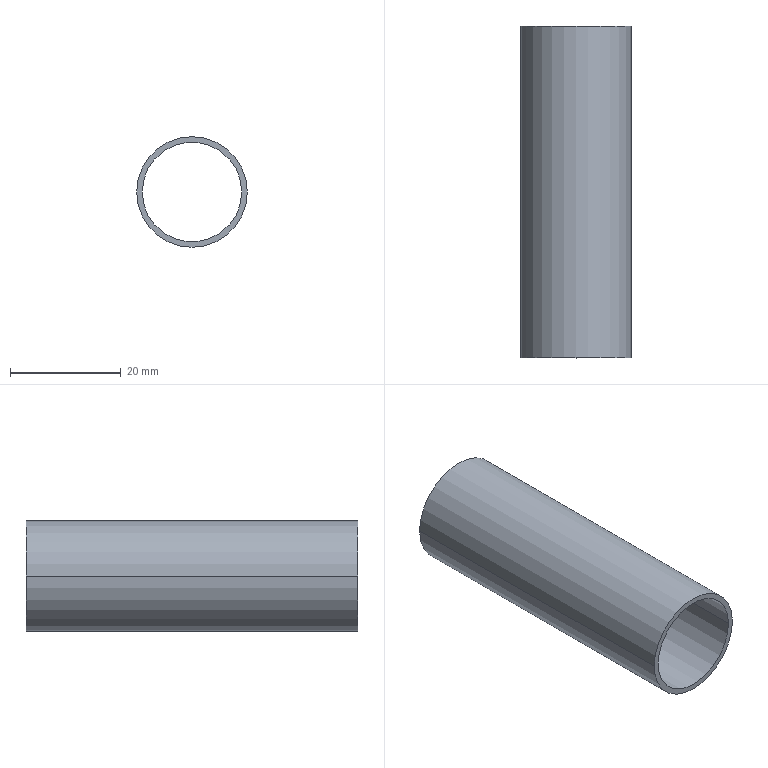Part | STEP file | A22NZ-A-301 | 1 solid | 6 faces | box 20 x 60 x 20 mm | volume 3581 mm3 | cylinder 4 | plane 2 | commonest cylinder face diameters 18 x2 20 x2
STEP:
#1=CARTESIAN_POINT('',(-10.,0.,0.));
#2=VERTEX_POINT('',#1);
#3=CARTESIAN_POINT('',(10.,0.,0.));
#4=VERTEX_POINT('',#3);
#5=CARTESIAN_POINT('',(0.,0.,0.));
#6=DIRECTION('',(0.,1.,0.));
#7=DIRECTION('',(-1.,0.,0.));
#8=AXIS2_PLACEMENT_3D('',#5,#6,#7);
#9=CIRCLE('',#8,10.);
#10=EDGE_CURVE('',#2,#4,#9,.T.);
#11=ORIENTED_EDGE('',*,*,#10,.T.);
#12=CARTESIAN_POINT('',(10.,60.,0.));
#13=VERTEX_POINT('',#12);
#14=CARTESIAN_POINT('',(10.,53.252,0.));
#15=DIRECTION('',(0.,1.,0.));
#16=VECTOR('',#15,1000.);
#17=LINE('',#14,#16);
#18=EDGE_CURVE('',#4,#13,#17,.T.);
#19=ORIENTED_EDGE('',*,*,#18,.T.);
#20=CARTESIAN_POINT('',(-10.,60.,0.));
#21=VERTEX_POINT('',#20);
#22=CARTESIAN_POINT('',(0.,60.,0.));
#23=DIRECTION('',(0.,1.,0.));
#24=DIRECTION('',(-1.,0.,0.));
#25=AXIS2_PLACEMENT_3D('',#22,#23,#24);
#26=CIRCLE('',#25,10.);
#27=EDGE_CURVE('',#21,#13,#26,.T.);
#28=ORIENTED_EDGE('',*,*,#27,.F.);
#29=CARTESIAN_POINT('',(-10.,53.252,0.));
#30=DIRECTION('',(0.,1.,0.));
#31=VECTOR('',#30,1000.);
#32=LINE('',#29,#31);
#33=EDGE_CURVE('',#2,#21,#32,.T.);
#34=ORIENTED_EDGE('',*,*,#33,.F.);
#35=EDGE_LOOP('',(#11,#19,#28,#34));
#36=FACE_OUTER_BOUND('',#35,.T.);
#37=CARTESIAN_POINT('',(0.,53.252,0.));
#38=DIRECTION('',(0.,1.,0.));
#39=DIRECTION('',(-1.,0.,0.));
#40=AXIS2_PLACEMENT_3D('',#37,#38,#39);
#41=CYLINDRICAL_SURFACE('',#40,10.);
#42=ADVANCED_FACE('',(#36),#41,.T.);
#43=CARTESIAN_POINT('',(9.,0.,0.));
#44=VERTEX_POINT('',#43);
#45=CARTESIAN_POINT('',(-9.,0.,0.));
#46=VERTEX_POINT('',#45);
#47=CARTESIAN_POINT('',(0.,0.,0.));
#48=DIRECTION('',(0.,1.,0.));
#49=DIRECTION('',(-1.,0.,0.));
#50=AXIS2_PLACEMENT_3D('',#47,#48,#49);
#51=CIRCLE('',#50,9.);
#52=EDGE_CURVE('',#44,#46,#51,.T.);
#53=ORIENTED_EDGE('',*,*,#52,.F.);
#54=CARTESIAN_POINT('',(9.,60.,0.));
#55=VERTEX_POINT('',#54);
#56=CARTESIAN_POINT('',(9.,53.252,0.));
#57=DIRECTION('',(0.,1.,0.));
#58=VECTOR('',#57,1000.);
#59=LINE('',#56,#58);
#60=EDGE_CURVE('',#44,#55,#59,.T.);
#61=ORIENTED_EDGE('',*,*,#60,.T.);
#62=CARTESIAN_POINT('',(-9.,60.,0.));
#63=VERTEX_POINT('',#62);
#64=CARTESIAN_POINT('',(0.,60.,0.));
#65=DIRECTION('',(0.,1.,0.));
#66=DIRECTION('',(-1.,0.,0.));
#67=AXIS2_PLACEMENT_3D('',#64,#65,#66);
#68=CIRCLE('',#67,9.);
#69=EDGE_CURVE('',#55,#63,#68,.T.);
#70=ORIENTED_EDGE('',*,*,#69,.T.);
#71=CARTESIAN_POINT('',(-9.,53.252,0.));
#72=DIRECTION('',(0.,1.,0.));
#73=VECTOR('',#72,1000.);
#74=LINE('',#71,#73);
#75=EDGE_CURVE('',#46,#63,#74,.T.);
#76=ORIENTED_EDGE('',*,*,#75,.F.);
#77=EDGE_LOOP('',(#53,#61,#70,#76));
#78=FACE_OUTER_BOUND('',#77,.T.);
#79=CARTESIAN_POINT('',(0.,53.252,0.));
#80=DIRECTION('',(0.,1.,0.));
#81=DIRECTION('',(-1.,0.,0.));
#82=AXIS2_PLACEMENT_3D('',#79,#80,#81);
#83=CYLINDRICAL_SURFACE('',#82,9.);
#84=ADVANCED_FACE('',(#78),#83,.F.);
#85=ORIENTED_EDGE('',*,*,#60,.F.);
#86=CARTESIAN_POINT('',(0.,0.,0.));
#87=DIRECTION('',(0.,1.,0.));
#88=DIRECTION('',(-1.,0.,0.));
#89=AXIS2_PLACEMENT_3D('',#86,#87,#88);
#90=CIRCLE('',#89,9.);
#91=EDGE_CURVE('',#46,#44,#90,.T.);
#92=ORIENTED_EDGE('',*,*,#91,.F.);
#93=ORIENTED_EDGE('',*,*,#75,.T.);
#94=CARTESIAN_POINT('',(0.,60.,0.));
#95=DIRECTION('',(0.,1.,0.));
#96=DIRECTION('',(-1.,0.,0.));
#97=AXIS2_PLACEMENT_3D('',#94,#95,#96);
#98=CIRCLE('',#97,9.);
#99=EDGE_CURVE('',#63,#55,#98,.T.);
#100=ORIENTED_EDGE('',*,*,#99,.T.);
#101=EDGE_LOOP('',(#85,#92,#93,#100));
#102=FACE_OUTER_BOUND('',#101,.T.);
#103=CARTESIAN_POINT('',(0.,53.252,0.));
#104=DIRECTION('',(0.,1.,0.));
#105=DIRECTION('',(-1.,0.,0.));
#106=AXIS2_PLACEMENT_3D('',#103,#104,#105);
#107=CYLINDRICAL_SURFACE('',#106,9.);
#108=ADVANCED_FACE('',(#102),#107,.F.);
#109=ORIENTED_EDGE('',*,*,#10,.F.);
#110=CARTESIAN_POINT('',(0.,0.,0.));
#111=DIRECTION('',(0.,1.,0.));
#112=DIRECTION('',(-1.,0.,0.));
#113=AXIS2_PLACEMENT_3D('',#110,#111,#112);
#114=CIRCLE('',#113,10.);
#115=EDGE_CURVE('',#4,#2,#114,.T.);
#116=ORIENTED_EDGE('',*,*,#115,.F.);
#117=EDGE_LOOP('',(#109,#116));
#118=FACE_OUTER_BOUND('',#117,.T.);
#119=ORIENTED_EDGE('',*,*,#91,.T.);
#120=ORIENTED_EDGE('',*,*,#52,.T.);
#121=EDGE_LOOP('',(#119,#120));
#122=FACE_BOUND('',#121,.T.);
#123=CARTESIAN_POINT('',(9.,0.,0.));
#124=DIRECTION('',(0.,1.,0.));
#125=DIRECTION('',(-1.,0.,0.));
#126=AXIS2_PLACEMENT_3D('',#123,#124,#125);
#127=PLANE('',#126);
#128=ADVANCED_FACE('',(#118,#122),#127,.F.);
#129=ORIENTED_EDGE('',*,*,#18,.F.);
#130=ORIENTED_EDGE('',*,*,#115,.T.);
#131=ORIENTED_EDGE('',*,*,#33,.T.);
#132=CARTESIAN_POINT('',(0.,60.,0.));
#133=DIRECTION('',(0.,1.,0.));
#134=DIRECTION('',(-1.,0.,0.));
#135=AXIS2_PLACEMENT_3D('',#132,#133,#134);
#136=CIRCLE('',#135,10.);
#137=EDGE_CURVE('',#13,#21,#136,.T.);
#138=ORIENTED_EDGE('',*,*,#137,.F.);
#139=EDGE_LOOP('',(#129,#130,#131,#138));
#140=FACE_OUTER_BOUND('',#139,.T.);
#141=CARTESIAN_POINT('',(0.,53.252,0.));
#142=DIRECTION('',(0.,1.,0.));
#143=DIRECTION('',(-1.,0.,0.));
#144=AXIS2_PLACEMENT_3D('',#141,#142,#143);
#145=CYLINDRICAL_SURFACE('',#144,10.);
#146=ADVANCED_FACE('',(#140),#145,.T.);
#147=ORIENTED_EDGE('',*,*,#99,.F.);
#148=ORIENTED_EDGE('',*,*,#69,.F.);
#149=EDGE_LOOP('',(#147,#148));
#150=FACE_BOUND('',#149,.T.);
#151=ORIENTED_EDGE('',*,*,#27,.T.);
#152=ORIENTED_EDGE('',*,*,#137,.T.);
#153=EDGE_LOOP('',(#151,#152));
#154=FACE_OUTER_BOUND('',#153,.T.);
#155=CARTESIAN_POINT('',(9.,60.,0.));
#156=DIRECTION('',(0.,-1.,0.));
#157=DIRECTION('',(1.,0.,0.));
#158=AXIS2_PLACEMENT_3D('',#155,#156,#157);
#159=PLANE('',#158);
#160=ADVANCED_FACE('',(#150,#154),#159,.F.);
#161=CLOSED_SHELL('',(#42,#84,#108,#128,#146,#160));
#162=MANIFOLD_SOLID_BREP('',#161);
#163=CARTESIAN_POINT('',(0.,0.,0.));
#164=DIRECTION('',(0.,0.,1.));
#165=DIRECTION('',(1.,0.,0.));
#166=AXIS2_PLACEMENT_3D('',#163,#164,#165);
#167=(LENGTH_UNIT()NAMED_UNIT(*)SI_UNIT(.MILLI.,.METRE.));
#168=UNCERTAINTY_MEASURE_WITH_UNIT(LENGTH_MEASURE(0.00001),#167,'','');
#169=(NAMED_UNIT(*)PLANE_ANGLE_UNIT()SI_UNIT($,.RADIAN.));
#170=(NAMED_UNIT(*)SI_UNIT($,.STERADIAN.)SOLID_ANGLE_UNIT());
#171=(GEOMETRIC_REPRESENTATION_CONTEXT(3)GLOBAL_UNCERTAINTY_ASSIGNED_CONTEXT((#168))GLOBAL_UNIT_ASSIGNED_CONTEXT((#167,#169,#170))REPRESENTATION_CONTEXT('',''));
#172=ADVANCED_BREP_SHAPE_REPRESENTATION('',(#162,#166),#171);